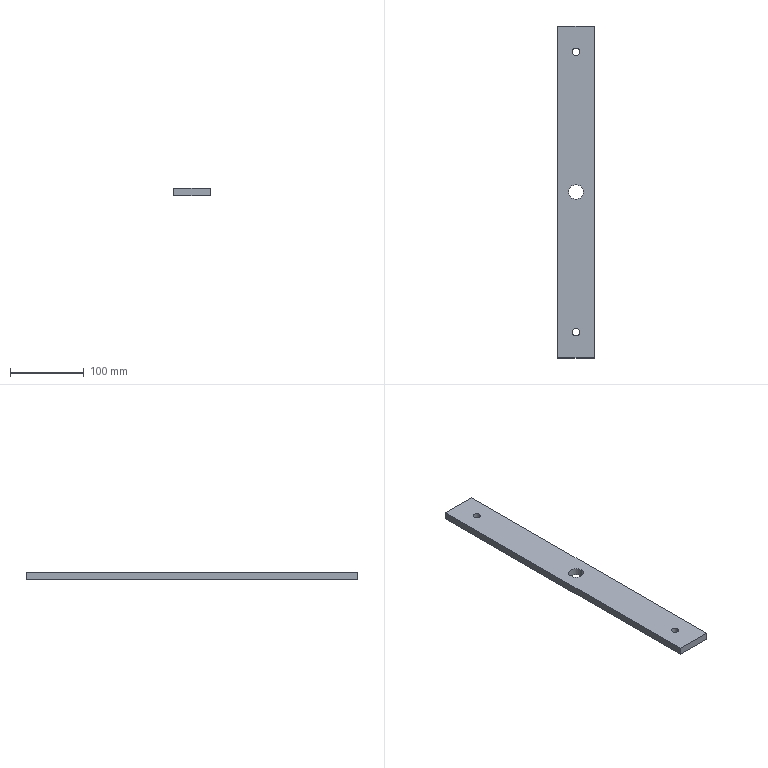Part | SolidWorks | features Extrusion 1 | 1 solid | 12 faces | box 50 x 450 x 10 mm | volume 220288 mm3 | cylinder 6 | plane 6 | commonest cylinder face diameters 10 x4 20 x2
STEP:
#1=CARTESIAN_POINT('',(20.,34.799,10.));
#2=VERTEX_POINT('',#1);
#3=CARTESIAN_POINT('',(30.,34.799,10.));
#4=VERTEX_POINT('',#3);
#5=CARTESIAN_POINT('',(25.,34.799,10.));
#6=DIRECTION('',(0.,0.,1.));
#7=DIRECTION('',(-1.,0.,0.));
#8=AXIS2_PLACEMENT_3D('',#5,#6,#7);
#9=CIRCLE('',#8,5.);
#10=EDGE_CURVE('',#2,#4,#9,.T.);
#11=ORIENTED_EDGE('',*,*,#10,.T.);
#12=CARTESIAN_POINT('',(30.,34.799,0.));
#13=VERTEX_POINT('',#12);
#14=CARTESIAN_POINT('',(30.,34.799,10.));
#15=DIRECTION('',(0.,0.,-1.));
#16=VECTOR('',#15,1000.);
#17=LINE('',#14,#16);
#18=EDGE_CURVE('',#4,#13,#17,.T.);
#19=ORIENTED_EDGE('',*,*,#18,.T.);
#20=CARTESIAN_POINT('',(20.,34.799,0.));
#21=VERTEX_POINT('',#20);
#22=CARTESIAN_POINT('',(25.,34.799,0.));
#23=DIRECTION('',(0.,0.,1.));
#24=DIRECTION('',(-1.,0.,0.));
#25=AXIS2_PLACEMENT_3D('',#22,#23,#24);
#26=CIRCLE('',#25,5.);
#27=EDGE_CURVE('',#21,#13,#26,.T.);
#28=ORIENTED_EDGE('',*,*,#27,.F.);
#29=CARTESIAN_POINT('',(20.,34.799,10.));
#30=DIRECTION('',(0.,0.,-1.));
#31=VECTOR('',#30,1000.);
#32=LINE('',#29,#31);
#33=EDGE_CURVE('',#2,#21,#32,.T.);
#34=ORIENTED_EDGE('',*,*,#33,.F.);
#35=EDGE_LOOP('',(#11,#19,#28,#34));
#36=FACE_OUTER_BOUND('',#35,.T.);
#37=CARTESIAN_POINT('',(25.,34.799,10.));
#38=DIRECTION('',(0.,0.,-1.));
#39=DIRECTION('',(-1.,0.,0.));
#40=AXIS2_PLACEMENT_3D('',#37,#38,#39);
#41=CYLINDRICAL_SURFACE('',#40,5.);
#42=ADVANCED_FACE('',(#36),#41,.F.);
#43=CARTESIAN_POINT('',(20.,415.201,10.));
#44=VERTEX_POINT('',#43);
#45=CARTESIAN_POINT('',(30.,415.201,10.));
#46=VERTEX_POINT('',#45);
#47=CARTESIAN_POINT('',(25.,415.201,10.));
#48=DIRECTION('',(0.,0.,1.));
#49=DIRECTION('',(1.,0.,0.));
#50=AXIS2_PLACEMENT_3D('',#47,#48,#49);
#51=CIRCLE('',#50,5.);
#52=EDGE_CURVE('',#44,#46,#51,.T.);
#53=ORIENTED_EDGE('',*,*,#52,.T.);
#54=CARTESIAN_POINT('',(30.,415.201,0.));
#55=VERTEX_POINT('',#54);
#56=CARTESIAN_POINT('',(30.,415.201,10.));
#57=DIRECTION('',(0.,0.,-1.));
#58=VECTOR('',#57,1000.);
#59=LINE('',#56,#58);
#60=EDGE_CURVE('',#46,#55,#59,.T.);
#61=ORIENTED_EDGE('',*,*,#60,.T.);
#62=CARTESIAN_POINT('',(20.,415.201,0.));
#63=VERTEX_POINT('',#62);
#64=CARTESIAN_POINT('',(25.,415.201,0.));
#65=DIRECTION('',(0.,0.,1.));
#66=DIRECTION('',(1.,0.,0.));
#67=AXIS2_PLACEMENT_3D('',#64,#65,#66);
#68=CIRCLE('',#67,5.);
#69=EDGE_CURVE('',#63,#55,#68,.T.);
#70=ORIENTED_EDGE('',*,*,#69,.F.);
#71=CARTESIAN_POINT('',(20.,415.201,10.));
#72=DIRECTION('',(0.,0.,-1.));
#73=VECTOR('',#72,1000.);
#74=LINE('',#71,#73);
#75=EDGE_CURVE('',#44,#63,#74,.T.);
#76=ORIENTED_EDGE('',*,*,#75,.F.);
#77=EDGE_LOOP('',(#53,#61,#70,#76));
#78=FACE_OUTER_BOUND('',#77,.T.);
#79=CARTESIAN_POINT('',(25.,415.201,10.));
#80=DIRECTION('',(0.,0.,-1.));
#81=DIRECTION('',(-1.,0.,0.));
#82=AXIS2_PLACEMENT_3D('',#79,#80,#81);
#83=CYLINDRICAL_SURFACE('',#82,5.);
#84=ADVANCED_FACE('',(#78),#83,.F.);
#85=CARTESIAN_POINT('',(15.,225.,10.));
#86=VERTEX_POINT('',#85);
#87=CARTESIAN_POINT('',(35.,225.,10.));
#88=VERTEX_POINT('',#87);
#89=CARTESIAN_POINT('',(25.,225.,10.));
#90=DIRECTION('',(0.,0.,1.));
#91=DIRECTION('',(1.,0.,0.));
#92=AXIS2_PLACEMENT_3D('',#89,#90,#91);
#93=CIRCLE('',#92,10.);
#94=EDGE_CURVE('',#86,#88,#93,.T.);
#95=ORIENTED_EDGE('',*,*,#94,.T.);
#96=CARTESIAN_POINT('',(35.,225.,0.));
#97=VERTEX_POINT('',#96);
#98=CARTESIAN_POINT('',(35.,225.,10.));
#99=DIRECTION('',(0.,0.,-1.));
#100=VECTOR('',#99,1000.);
#101=LINE('',#98,#100);
#102=EDGE_CURVE('',#88,#97,#101,.T.);
#103=ORIENTED_EDGE('',*,*,#102,.T.);
#104=CARTESIAN_POINT('',(15.,225.,0.));
#105=VERTEX_POINT('',#104);
#106=CARTESIAN_POINT('',(25.,225.,0.));
#107=DIRECTION('',(0.,0.,1.));
#108=DIRECTION('',(1.,0.,0.));
#109=AXIS2_PLACEMENT_3D('',#106,#107,#108);
#110=CIRCLE('',#109,10.);
#111=EDGE_CURVE('',#105,#97,#110,.T.);
#112=ORIENTED_EDGE('',*,*,#111,.F.);
#113=CARTESIAN_POINT('',(15.,225.,10.));
#114=DIRECTION('',(0.,0.,-1.));
#115=VECTOR('',#114,1000.);
#116=LINE('',#113,#115);
#117=EDGE_CURVE('',#86,#105,#116,.T.);
#118=ORIENTED_EDGE('',*,*,#117,.F.);
#119=EDGE_LOOP('',(#95,#103,#112,#118));
#120=FACE_OUTER_BOUND('',#119,.T.);
#121=CARTESIAN_POINT('',(25.,225.,10.));
#122=DIRECTION('',(0.,0.,-1.));
#123=DIRECTION('',(-1.,0.,0.));
#124=AXIS2_PLACEMENT_3D('',#121,#122,#123);
#125=CYLINDRICAL_SURFACE('',#124,10.);
#126=ADVANCED_FACE('',(#120),#125,.F.);
#127=CARTESIAN_POINT('',(0.,0.,10.));
#128=VERTEX_POINT('',#127);
#129=CARTESIAN_POINT('',(50.,0.,10.));
#130=VERTEX_POINT('',#129);
#131=CARTESIAN_POINT('',(50.,0.,10.));
#132=DIRECTION('',(1.,0.,0.));
#133=VECTOR('',#132,1000.);
#134=LINE('',#131,#133);
#135=EDGE_CURVE('',#128,#130,#134,.T.);
#136=ORIENTED_EDGE('',*,*,#135,.T.);
#137=CARTESIAN_POINT('',(50.,450.,10.));
#138=VERTEX_POINT('',#137);
#139=CARTESIAN_POINT('',(50.,450.,10.));
#140=DIRECTION('',(0.,1.,0.));
#141=VECTOR('',#140,1000.);
#142=LINE('',#139,#141);
#143=EDGE_CURVE('',#130,#138,#142,.T.);
#144=ORIENTED_EDGE('',*,*,#143,.T.);
#145=CARTESIAN_POINT('',(0.,450.,10.));
#146=VERTEX_POINT('',#145);
#147=CARTESIAN_POINT('',(0.,450.,10.));
#148=DIRECTION('',(-1.,0.,0.));
#149=VECTOR('',#148,1000.);
#150=LINE('',#147,#149);
#151=EDGE_CURVE('',#138,#146,#150,.T.);
#152=ORIENTED_EDGE('',*,*,#151,.T.);
#153=CARTESIAN_POINT('',(0.,0.,10.));
#154=DIRECTION('',(0.,-1.,0.));
#155=VECTOR('',#154,1000.);
#156=LINE('',#153,#155);
#157=EDGE_CURVE('',#146,#128,#156,.T.);
#158=ORIENTED_EDGE('',*,*,#157,.T.);
#159=EDGE_LOOP('',(#136,#144,#152,#158));
#160=FACE_OUTER_BOUND('',#159,.T.);
#161=ORIENTED_EDGE('',*,*,#94,.F.);
#162=CARTESIAN_POINT('',(25.,225.,10.));
#163=DIRECTION('',(0.,0.,1.));
#164=DIRECTION('',(1.,0.,0.));
#165=AXIS2_PLACEMENT_3D('',#162,#163,#164);
#166=CIRCLE('',#165,10.);
#167=EDGE_CURVE('',#88,#86,#166,.T.);
#168=ORIENTED_EDGE('',*,*,#167,.F.);
#169=EDGE_LOOP('',(#161,#168));
#170=FACE_BOUND('',#169,.T.);
#171=ORIENTED_EDGE('',*,*,#52,.F.);
#172=CARTESIAN_POINT('',(25.,415.201,10.));
#173=DIRECTION('',(0.,0.,1.));
#174=DIRECTION('',(1.,0.,0.));
#175=AXIS2_PLACEMENT_3D('',#172,#173,#174);
#176=CIRCLE('',#175,5.);
#177=EDGE_CURVE('',#46,#44,#176,.T.);
#178=ORIENTED_EDGE('',*,*,#177,.F.);
#179=EDGE_LOOP('',(#171,#178));
#180=FACE_BOUND('',#179,.T.);
#181=ORIENTED_EDGE('',*,*,#10,.F.);
#182=CARTESIAN_POINT('',(25.,34.799,10.));
#183=DIRECTION('',(0.,0.,1.));
#184=DIRECTION('',(-1.,0.,0.));
#185=AXIS2_PLACEMENT_3D('',#182,#183,#184);
#186=CIRCLE('',#185,5.);
#187=EDGE_CURVE('',#4,#2,#186,.T.);
#188=ORIENTED_EDGE('',*,*,#187,.F.);
#189=EDGE_LOOP('',(#181,#188));
#190=FACE_BOUND('',#189,.T.);
#191=CARTESIAN_POINT('',(0.,0.,10.));
#192=DIRECTION('',(0.,0.,-1.));
#193=DIRECTION('',(-1.,0.,0.));
#194=AXIS2_PLACEMENT_3D('',#191,#192,#193);
#195=PLANE('',#194);
#196=ADVANCED_FACE('',(#160,#170,#180,#190),#195,.F.);
#197=ORIENTED_EDGE('',*,*,#69,.T.);
#198=CARTESIAN_POINT('',(25.,415.201,0.));
#199=DIRECTION('',(0.,0.,1.));
#200=DIRECTION('',(1.,0.,0.));
#201=AXIS2_PLACEMENT_3D('',#198,#199,#200);
#202=CIRCLE('',#201,5.);
#203=EDGE_CURVE('',#55,#63,#202,.T.);
#204=ORIENTED_EDGE('',*,*,#203,.T.);
#205=EDGE_LOOP('',(#197,#204));
#206=FACE_BOUND('',#205,.T.);
#207=CARTESIAN_POINT('',(0.,0.,0.));
#208=VERTEX_POINT('',#207);
#209=CARTESIAN_POINT('',(50.,0.,0.));
#210=VERTEX_POINT('',#209);
#211=CARTESIAN_POINT('',(50.,0.,0.));
#212=DIRECTION('',(1.,0.,0.));
#213=VECTOR('',#212,1000.);
#214=LINE('',#211,#213);
#215=EDGE_CURVE('',#208,#210,#214,.T.);
#216=ORIENTED_EDGE('',*,*,#215,.F.);
#217=CARTESIAN_POINT('',(0.,450.,0.));
#218=VERTEX_POINT('',#217);
#219=CARTESIAN_POINT('',(0.,0.,0.));
#220=DIRECTION('',(0.,-1.,0.));
#221=VECTOR('',#220,1000.);
#222=LINE('',#219,#221);
#223=EDGE_CURVE('',#218,#208,#222,.T.);
#224=ORIENTED_EDGE('',*,*,#223,.F.);
#225=CARTESIAN_POINT('',(50.,450.,0.));
#226=VERTEX_POINT('',#225);
#227=CARTESIAN_POINT('',(0.,450.,0.));
#228=DIRECTION('',(-1.,0.,0.));
#229=VECTOR('',#228,1000.);
#230=LINE('',#227,#229);
#231=EDGE_CURVE('',#226,#218,#230,.T.);
#232=ORIENTED_EDGE('',*,*,#231,.F.);
#233=CARTESIAN_POINT('',(50.,450.,0.));
#234=DIRECTION('',(0.,1.,0.));
#235=VECTOR('',#234,1000.);
#236=LINE('',#233,#235);
#237=EDGE_CURVE('',#210,#226,#236,.T.);
#238=ORIENTED_EDGE('',*,*,#237,.F.);
#239=EDGE_LOOP('',(#216,#224,#232,#238));
#240=FACE_OUTER_BOUND('',#239,.T.);
#241=ORIENTED_EDGE('',*,*,#111,.T.);
#242=CARTESIAN_POINT('',(25.,225.,0.));
#243=DIRECTION('',(0.,0.,1.));
#244=DIRECTION('',(1.,0.,0.));
#245=AXIS2_PLACEMENT_3D('',#242,#243,#244);
#246=CIRCLE('',#245,10.);
#247=EDGE_CURVE('',#97,#105,#246,.T.);
#248=ORIENTED_EDGE('',*,*,#247,.T.);
#249=EDGE_LOOP('',(#241,#248));
#250=FACE_BOUND('',#249,.T.);
#251=ORIENTED_EDGE('',*,*,#27,.T.);
#252=CARTESIAN_POINT('',(25.,34.799,0.));
#253=DIRECTION('',(0.,0.,1.));
#254=DIRECTION('',(-1.,0.,0.));
#255=AXIS2_PLACEMENT_3D('',#252,#253,#254);
#256=CIRCLE('',#255,5.);
#257=EDGE_CURVE('',#13,#21,#256,.T.);
#258=ORIENTED_EDGE('',*,*,#257,.T.);
#259=EDGE_LOOP('',(#251,#258));
#260=FACE_BOUND('',#259,.T.);
#261=CARTESIAN_POINT('',(0.,0.,0.));
#262=DIRECTION('',(0.,0.,-1.));
#263=DIRECTION('',(-1.,0.,0.));
#264=AXIS2_PLACEMENT_3D('',#261,#262,#263);
#265=PLANE('',#264);
#266=ADVANCED_FACE('',(#206,#240,#250,#260),#265,.T.);
#267=ORIENTED_EDGE('',*,*,#215,.T.);
#268=CARTESIAN_POINT('',(50.,0.,10.));
#269=DIRECTION('',(0.,0.,-1.));
#270=VECTOR('',#269,1000.);
#271=LINE('',#268,#270);
#272=EDGE_CURVE('',#130,#210,#271,.T.);
#273=ORIENTED_EDGE('',*,*,#272,.F.);
#274=ORIENTED_EDGE('',*,*,#135,.F.);
#275=CARTESIAN_POINT('',(0.,0.,10.));
#276=DIRECTION('',(0.,0.,-1.));
#277=VECTOR('',#276,1000.);
#278=LINE('',#275,#277);
#279=EDGE_CURVE('',#128,#208,#278,.T.);
#280=ORIENTED_EDGE('',*,*,#279,.T.);
#281=EDGE_LOOP('',(#267,#273,#274,#280));
#282=FACE_OUTER_BOUND('',#281,.T.);
#283=CARTESIAN_POINT('',(50.,0.,10.));
#284=DIRECTION('',(0.,1.,0.));
#285=DIRECTION('',(0.,0.,1.));
#286=AXIS2_PLACEMENT_3D('',#283,#284,#285);
#287=PLANE('',#286);
#288=ADVANCED_FACE('',(#282),#287,.F.);
#289=ORIENTED_EDGE('',*,*,#237,.T.);
#290=CARTESIAN_POINT('',(50.,450.,10.));
#291=DIRECTION('',(0.,0.,-1.));
#292=VECTOR('',#291,1000.);
#293=LINE('',#290,#292);
#294=EDGE_CURVE('',#138,#226,#293,.T.);
#295=ORIENTED_EDGE('',*,*,#294,.F.);
#296=ORIENTED_EDGE('',*,*,#143,.F.);
#297=ORIENTED_EDGE('',*,*,#272,.T.);
#298=EDGE_LOOP('',(#289,#295,#296,#297));
#299=FACE_OUTER_BOUND('',#298,.T.);
#300=CARTESIAN_POINT('',(50.,450.,10.));
#301=DIRECTION('',(-1.,0.,0.));
#302=DIRECTION('',(0.,-1.,0.));
#303=AXIS2_PLACEMENT_3D('',#300,#301,#302);
#304=PLANE('',#303);
#305=ADVANCED_FACE('',(#299),#304,.F.);
#306=ORIENTED_EDGE('',*,*,#231,.T.);
#307=CARTESIAN_POINT('',(0.,450.,10.));
#308=DIRECTION('',(0.,0.,-1.));
#309=VECTOR('',#308,1000.);
#310=LINE('',#307,#309);
#311=EDGE_CURVE('',#146,#218,#310,.T.);
#312=ORIENTED_EDGE('',*,*,#311,.F.);
#313=ORIENTED_EDGE('',*,*,#151,.F.);
#314=ORIENTED_EDGE('',*,*,#294,.T.);
#315=EDGE_LOOP('',(#306,#312,#313,#314));
#316=FACE_OUTER_BOUND('',#315,.T.);
#317=CARTESIAN_POINT('',(0.,450.,10.));
#318=DIRECTION('',(0.,-1.,0.));
#319=DIRECTION('',(0.,0.,-1.));
#320=AXIS2_PLACEMENT_3D('',#317,#318,#319);
#321=PLANE('',#320);
#322=ADVANCED_FACE('',(#316),#321,.F.);
#323=ORIENTED_EDGE('',*,*,#223,.T.);
#324=ORIENTED_EDGE('',*,*,#279,.F.);
#325=ORIENTED_EDGE('',*,*,#157,.F.);
#326=ORIENTED_EDGE('',*,*,#311,.T.);
#327=EDGE_LOOP('',(#323,#324,#325,#326));
#328=FACE_OUTER_BOUND('',#327,.T.);
#329=CARTESIAN_POINT('',(0.,0.,10.));
#330=DIRECTION('',(1.,0.,0.));
#331=DIRECTION('',(0.,1.,0.));
#332=AXIS2_PLACEMENT_3D('',#329,#330,#331);
#333=PLANE('',#332);
#334=ADVANCED_FACE('',(#328),#333,.F.);
#335=ORIENTED_EDGE('',*,*,#102,.F.);
#336=ORIENTED_EDGE('',*,*,#167,.T.);
#337=ORIENTED_EDGE('',*,*,#117,.T.);
#338=ORIENTED_EDGE('',*,*,#247,.F.);
#339=EDGE_LOOP('',(#335,#336,#337,#338));
#340=FACE_OUTER_BOUND('',#339,.T.);
#341=CARTESIAN_POINT('',(25.,225.,10.));
#342=DIRECTION('',(0.,0.,-1.));
#343=DIRECTION('',(-1.,0.,0.));
#344=AXIS2_PLACEMENT_3D('',#341,#342,#343);
#345=CYLINDRICAL_SURFACE('',#344,10.);
#346=ADVANCED_FACE('',(#340),#345,.F.);
#347=ORIENTED_EDGE('',*,*,#60,.F.);
#348=ORIENTED_EDGE('',*,*,#177,.T.);
#349=ORIENTED_EDGE('',*,*,#75,.T.);
#350=ORIENTED_EDGE('',*,*,#203,.F.);
#351=EDGE_LOOP('',(#347,#348,#349,#350));
#352=FACE_OUTER_BOUND('',#351,.T.);
#353=CARTESIAN_POINT('',(25.,415.201,10.));
#354=DIRECTION('',(0.,0.,-1.));
#355=DIRECTION('',(-1.,0.,0.));
#356=AXIS2_PLACEMENT_3D('',#353,#354,#355);
#357=CYLINDRICAL_SURFACE('',#356,5.);
#358=ADVANCED_FACE('',(#352),#357,.F.);
#359=ORIENTED_EDGE('',*,*,#18,.F.);
#360=ORIENTED_EDGE('',*,*,#187,.T.);
#361=ORIENTED_EDGE('',*,*,#33,.T.);
#362=ORIENTED_EDGE('',*,*,#257,.F.);
#363=EDGE_LOOP('',(#359,#360,#361,#362));
#364=FACE_OUTER_BOUND('',#363,.T.);
#365=CARTESIAN_POINT('',(25.,34.799,10.));
#366=DIRECTION('',(0.,0.,-1.));
#367=DIRECTION('',(-1.,0.,0.));
#368=AXIS2_PLACEMENT_3D('',#365,#366,#367);
#369=CYLINDRICAL_SURFACE('',#368,5.);
#370=ADVANCED_FACE('',(#364),#369,.F.);
#371=CLOSED_SHELL('',(#42,#84,#126,#196,#266,#288,#305,#322,#334,#346,#358,#370));
#372=MANIFOLD_SOLID_BREP('',#371);
#373=CARTESIAN_POINT('',(0.,0.,0.));
#374=DIRECTION('',(0.,0.,1.));
#375=DIRECTION('',(1.,0.,0.));
#376=AXIS2_PLACEMENT_3D('',#373,#374,#375);
#377=(LENGTH_UNIT()NAMED_UNIT(*)SI_UNIT(.MILLI.,.METRE.));
#378=UNCERTAINTY_MEASURE_WITH_UNIT(LENGTH_MEASURE(0.00001),#377,'','');
#379=(NAMED_UNIT(*)PLANE_ANGLE_UNIT()SI_UNIT($,.RADIAN.));
#380=(NAMED_UNIT(*)SI_UNIT($,.STERADIAN.)SOLID_ANGLE_UNIT());
#381=(GEOMETRIC_REPRESENTATION_CONTEXT(3)GLOBAL_UNCERTAINTY_ASSIGNED_CONTEXT((#378))GLOBAL_UNIT_ASSIGNED_CONTEXT((#377,#379,#380))REPRESENTATION_CONTEXT('',''));
#382=ADVANCED_BREP_SHAPE_REPRESENTATION('',(#372,#376),#381);